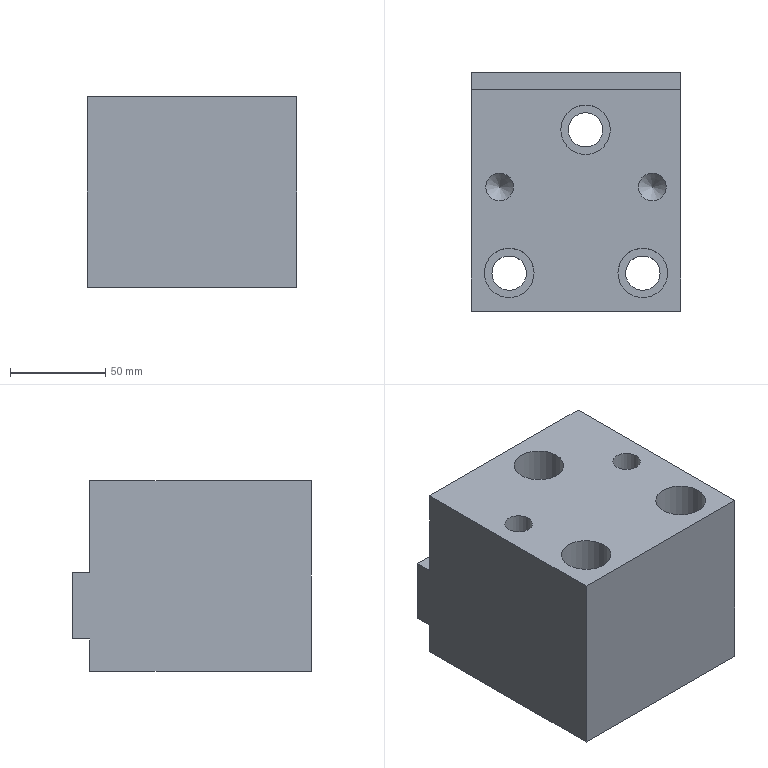Part | STEP file | lll_id4722_x_t | 1 solid | 27 faces | box 110 x 125 x 100 mm | volume 1169474 mm3 | plane 13 | cylinder 10 | cone 4 | commonest cylinder face diameters 18.009 x3 26.008 x3 8.5 x2 14.506 x2
STEP:
#1=CARTESIAN_POINT('',(1322.592,-417.359,5.));
#2=VERTEX_POINT('',#1);
#3=CARTESIAN_POINT('',(1315.339,-417.359,5.));
#4=DIRECTION('',(0.,0.,1.));
#5=DIRECTION('',(1.,0.,0.));
#6=AXIS2_PLACEMENT_3D('',#3,#4,#5);
#7=CIRCLE('',#6,7.253);
#8=EDGE_CURVE('',#2,#2,#7,.T.);
#9=ORIENTED_EDGE('',*,*,#8,.F.);
#10=EDGE_LOOP('',(#9));
#11=FACE_BOUND('',#10,.T.);
#12=CARTESIAN_POINT('',(1402.592,-417.359,5.));
#13=VERTEX_POINT('',#12);
#14=CARTESIAN_POINT('',(1395.339,-417.359,5.));
#15=DIRECTION('',(0.,0.,1.));
#16=DIRECTION('',(1.,0.,0.));
#17=AXIS2_PLACEMENT_3D('',#14,#15,#16);
#18=CIRCLE('',#17,7.253);
#19=EDGE_CURVE('',#13,#13,#18,.T.);
#20=ORIENTED_EDGE('',*,*,#19,.F.);
#21=EDGE_LOOP('',(#20));
#22=FACE_BOUND('',#21,.T.);
#23=CARTESIAN_POINT('',(1300.339,-366.359,5.));
#24=VERTEX_POINT('',#23);
#25=CARTESIAN_POINT('',(1410.339,-366.359,5.));
#26=VERTEX_POINT('',#25);
#27=CARTESIAN_POINT('',(-3297.001,-366.359,5.));
#28=DIRECTION('',(1.,0.,0.));
#29=VECTOR('',#28,1.);
#30=LINE('',#27,#29);
#31=EDGE_CURVE('',#24,#26,#30,.T.);
#32=ORIENTED_EDGE('',*,*,#31,.F.);
#33=CARTESIAN_POINT('',(1300.339,-482.359,5.));
#34=VERTEX_POINT('',#33);
#35=CARTESIAN_POINT('',(1300.339,-382.359,5.));
#36=DIRECTION('',(0.,-1.,0.));
#37=VECTOR('',#36,1.);
#38=LINE('',#35,#37);
#39=EDGE_CURVE('',#24,#34,#38,.T.);
#40=ORIENTED_EDGE('',*,*,#39,.T.);
#41=CARTESIAN_POINT('',(1410.339,-482.359,5.));
#42=VERTEX_POINT('',#41);
#43=CARTESIAN_POINT('',(1308.588,-482.359,5.));
#44=DIRECTION('',(-1.,0.,0.));
#45=VECTOR('',#44,1.);
#46=LINE('',#43,#45);
#47=EDGE_CURVE('',#42,#34,#46,.T.);
#48=ORIENTED_EDGE('',*,*,#47,.F.);
#49=CARTESIAN_POINT('',(1410.339,-382.359,5.));
#50=DIRECTION('',(0.,1.,0.));
#51=VECTOR('',#50,1.);
#52=LINE('',#49,#51);
#53=EDGE_CURVE('',#42,#26,#52,.T.);
#54=ORIENTED_EDGE('',*,*,#53,.T.);
#55=EDGE_LOOP('',(#32,#40,#48,#54));
#56=FACE_BOUND('',#55,.T.);
#57=CARTESIAN_POINT('',(1377.335,-462.359,5.));
#58=VERTEX_POINT('',#57);
#59=CARTESIAN_POINT('',(1390.339,-462.359,5.));
#60=DIRECTION('',(0.,0.,1.));
#61=DIRECTION('',(-1.,0.,0.));
#62=AXIS2_PLACEMENT_3D('',#59,#60,#61);
#63=CIRCLE('',#62,13.004);
#64=EDGE_CURVE('',#58,#58,#63,.T.);
#65=ORIENTED_EDGE('',*,*,#64,.F.);
#66=EDGE_LOOP('',(#65));
#67=FACE_BOUND('',#66,.T.);
#68=CARTESIAN_POINT('',(1307.335,-462.359,5.));
#69=VERTEX_POINT('',#68);
#70=CARTESIAN_POINT('',(1320.339,-462.359,5.));
#71=DIRECTION('',(0.,0.,1.));
#72=DIRECTION('',(-1.,0.,0.));
#73=AXIS2_PLACEMENT_3D('',#70,#71,#72);
#74=CIRCLE('',#73,13.004);
#75=EDGE_CURVE('',#69,#69,#74,.T.);
#76=ORIENTED_EDGE('',*,*,#75,.F.);
#77=EDGE_LOOP('',(#76));
#78=FACE_BOUND('',#77,.T.);
#79=CARTESIAN_POINT('',(1373.343,-387.359,5.));
#80=VERTEX_POINT('',#79);
#81=CARTESIAN_POINT('',(1360.339,-387.359,5.));
#82=DIRECTION('',(0.,0.,-1.));
#83=DIRECTION('',(1.,0.,0.));
#84=AXIS2_PLACEMENT_3D('',#81,#82,#83);
#85=CIRCLE('',#84,13.004);
#86=EDGE_CURVE('',#80,#80,#85,.T.);
#87=ORIENTED_EDGE('',*,*,#86,.T.);
#88=EDGE_LOOP('',(#87));
#89=FACE_BOUND('',#88,.T.);
#90=CARTESIAN_POINT('',(1308.588,-382.359,5.));
#91=DIRECTION('',(0.,0.,-1.));
#92=DIRECTION('',(1.,0.,0.));
#93=AXIS2_PLACEMENT_3D('',#90,#91,#92);
#94=PLANE('',#93);
#95=ADVANCED_FACE('',(#11,#22,#56,#67,#78,#89),#94,.F.);
#96=CARTESIAN_POINT('',(1330.339,-366.359,-23.25));
#97=VERTEX_POINT('',#96);
#98=CARTESIAN_POINT('',(1330.339,-366.359,-19.));
#99=DIRECTION('',(0.,-1.,0.));
#100=DIRECTION('',(0.,0.,-1.));
#101=AXIS2_PLACEMENT_3D('',#98,#99,#100);
#102=CIRCLE('',#101,4.25);
#103=EDGE_CURVE('',#97,#97,#102,.T.);
#104=ORIENTED_EDGE('',*,*,#103,.T.);
#105=EDGE_LOOP('',(#104));
#106=FACE_BOUND('',#105,.T.);
#107=CARTESIAN_POINT('',(1380.339,-366.359,-23.25));
#108=VERTEX_POINT('',#107);
#109=CARTESIAN_POINT('',(1380.339,-366.359,-19.));
#110=DIRECTION('',(0.,-1.,0.));
#111=DIRECTION('',(0.,0.,-1.));
#112=AXIS2_PLACEMENT_3D('',#109,#110,#111);
#113=CIRCLE('',#112,4.25);
#114=EDGE_CURVE('',#108,#108,#113,.T.);
#115=ORIENTED_EDGE('',*,*,#114,.T.);
#116=EDGE_LOOP('',(#115));
#117=FACE_BOUND('',#116,.T.);
#118=CARTESIAN_POINT('',(1300.339,-366.359,-43.));
#119=VERTEX_POINT('',#118);
#120=CARTESIAN_POINT('',(1410.339,-366.359,-43.));
#121=VERTEX_POINT('',#120);
#122=CARTESIAN_POINT('',(1305.339,-366.359,-43.));
#123=DIRECTION('',(1.,0.,0.));
#124=VECTOR('',#123,1.);
#125=LINE('',#122,#124);
#126=EDGE_CURVE('',#119,#121,#125,.T.);
#127=ORIENTED_EDGE('',*,*,#126,.F.);
#128=CARTESIAN_POINT('',(1300.339,-366.359,-625.));
#129=DIRECTION('',(0.,0.,-1.));
#130=VECTOR('',#129,1.);
#131=LINE('',#128,#130);
#132=EDGE_CURVE('',#24,#119,#131,.T.);
#133=ORIENTED_EDGE('',*,*,#132,.F.);
#134=ORIENTED_EDGE('',*,*,#31,.T.);
#135=CARTESIAN_POINT('',(1410.339,-366.359,-35.));
#136=DIRECTION('',(0.,0.,1.));
#137=VECTOR('',#136,1.);
#138=LINE('',#135,#137);
#139=EDGE_CURVE('',#121,#26,#138,.T.);
#140=ORIENTED_EDGE('',*,*,#139,.F.);
#141=EDGE_LOOP('',(#127,#133,#134,#140));
#142=FACE_BOUND('',#141,.T.);
#143=CARTESIAN_POINT('',(-3297.001,-366.359,-625.));
#144=DIRECTION('',(0.,1.,0.));
#145=DIRECTION('',(0.,0.,1.));
#146=AXIS2_PLACEMENT_3D('',#143,#144,#145);
#147=PLANE('',#146);
#148=ADVANCED_FACE('',(#106,#117,#142),#147,.T.);
#149=CARTESIAN_POINT('',(1300.339,-357.359,-78.));
#150=VERTEX_POINT('',#149);
#151=CARTESIAN_POINT('',(1300.339,-366.359,-78.));
#152=VERTEX_POINT('',#151);
#153=CARTESIAN_POINT('',(1300.339,-407.359,-78.));
#154=DIRECTION('',(0.,-1.,0.));
#155=VECTOR('',#154,1.);
#156=LINE('',#153,#155);
#157=EDGE_CURVE('',#150,#152,#156,.T.);
#158=ORIENTED_EDGE('',*,*,#157,.T.);
#159=CARTESIAN_POINT('',(1300.339,-366.359,-95.));
#160=VERTEX_POINT('',#159);
#161=CARTESIAN_POINT('',(1300.339,-366.359,72.5));
#162=DIRECTION('',(0.,0.,-1.));
#163=VECTOR('',#162,1.);
#164=LINE('',#161,#163);
#165=EDGE_CURVE('',#152,#160,#164,.T.);
#166=ORIENTED_EDGE('',*,*,#165,.T.);
#167=CARTESIAN_POINT('',(1300.339,-482.359,-95.));
#168=VERTEX_POINT('',#167);
#169=CARTESIAN_POINT('',(1300.339,-407.359,-95.));
#170=DIRECTION('',(0.,1.,0.));
#171=VECTOR('',#170,1.);
#172=LINE('',#169,#171);
#173=EDGE_CURVE('',#168,#160,#172,.T.);
#174=ORIENTED_EDGE('',*,*,#173,.F.);
#175=CARTESIAN_POINT('',(1300.339,-482.359,-650.));
#176=DIRECTION('',(0.,0.,-1.));
#177=VECTOR('',#176,1.);
#178=LINE('',#175,#177);
#179=EDGE_CURVE('',#34,#168,#178,.T.);
#180=ORIENTED_EDGE('',*,*,#179,.F.);
#181=ORIENTED_EDGE('',*,*,#39,.F.);
#182=ORIENTED_EDGE('',*,*,#132,.T.);
#183=CARTESIAN_POINT('',(1300.339,-357.359,-43.));
#184=VERTEX_POINT('',#183);
#185=CARTESIAN_POINT('',(1300.339,-397.359,-43.));
#186=DIRECTION('',(0.,1.,0.));
#187=VECTOR('',#186,1.);
#188=LINE('',#185,#187);
#189=EDGE_CURVE('',#119,#184,#188,.T.);
#190=ORIENTED_EDGE('',*,*,#189,.T.);
#191=CARTESIAN_POINT('',(1300.339,-357.359,72.5));
#192=DIRECTION('',(0.,0.,-1.));
#193=VECTOR('',#192,1.);
#194=LINE('',#191,#193);
#195=EDGE_CURVE('',#184,#150,#194,.T.);
#196=ORIENTED_EDGE('',*,*,#195,.T.);
#197=EDGE_LOOP('',(#158,#166,#174,#180,#181,#182,#190,#196));
#198=FACE_OUTER_BOUND('',#197,.T.);
#199=CARTESIAN_POINT('',(1300.339,-407.359,72.5));
#200=DIRECTION('',(-1.,0.,0.));
#201=DIRECTION('',(0.,0.,-1.));
#202=AXIS2_PLACEMENT_3D('',#199,#200,#201);
#203=PLANE('',#202);
#204=ADVANCED_FACE('',(#198),#203,.T.);
#205=CARTESIAN_POINT('',(1410.339,-357.359,-78.));
#206=VERTEX_POINT('',#205);
#207=CARTESIAN_POINT('',(-3297.001,-357.359,-78.));
#208=DIRECTION('',(1.,0.,0.));
#209=VECTOR('',#208,1.);
#210=LINE('',#207,#209);
#211=EDGE_CURVE('',#150,#206,#210,.T.);
#212=ORIENTED_EDGE('',*,*,#211,.F.);
#213=ORIENTED_EDGE('',*,*,#195,.F.);
#214=CARTESIAN_POINT('',(1410.339,-357.359,-43.));
#215=VERTEX_POINT('',#214);
#216=CARTESIAN_POINT('',(-3297.001,-357.359,-43.));
#217=DIRECTION('',(-1.,0.,0.));
#218=VECTOR('',#217,1.);
#219=LINE('',#216,#218);
#220=EDGE_CURVE('',#215,#184,#219,.T.);
#221=ORIENTED_EDGE('',*,*,#220,.F.);
#222=CARTESIAN_POINT('',(1410.339,-357.359,-60.));
#223=DIRECTION('',(0.,0.,1.));
#224=VECTOR('',#223,1.);
#225=LINE('',#222,#224);
#226=EDGE_CURVE('',#206,#215,#225,.T.);
#227=ORIENTED_EDGE('',*,*,#226,.F.);
#228=EDGE_LOOP('',(#212,#213,#221,#227));
#229=FACE_OUTER_BOUND('',#228,.T.);
#230=CARTESIAN_POINT('',(-3297.001,-357.359,-650.));
#231=DIRECTION('',(0.,1.,0.));
#232=DIRECTION('',(0.,0.,1.));
#233=AXIS2_PLACEMENT_3D('',#230,#231,#232);
#234=PLANE('',#233);
#235=ADVANCED_FACE('',(#229),#234,.T.);
#236=ORIENTED_EDGE('',*,*,#179,.T.);
#237=CARTESIAN_POINT('',(1410.339,-482.359,-95.));
#238=VERTEX_POINT('',#237);
#239=CARTESIAN_POINT('',(-3297.001,-482.359,-95.));
#240=DIRECTION('',(1.,0.,0.));
#241=VECTOR('',#240,1.);
#242=LINE('',#239,#241);
#243=EDGE_CURVE('',#168,#238,#242,.T.);
#244=ORIENTED_EDGE('',*,*,#243,.T.);
#245=CARTESIAN_POINT('',(1410.339,-482.359,-650.));
#246=DIRECTION('',(0.,0.,-1.));
#247=VECTOR('',#246,1.);
#248=LINE('',#245,#247);
#249=EDGE_CURVE('',#42,#238,#248,.T.);
#250=ORIENTED_EDGE('',*,*,#249,.F.);
#251=ORIENTED_EDGE('',*,*,#47,.T.);
#252=EDGE_LOOP('',(#236,#244,#250,#251));
#253=FACE_OUTER_BOUND('',#252,.T.);
#254=CARTESIAN_POINT('',(-3297.001,-482.359,-650.));
#255=DIRECTION('',(0.,1.,0.));
#256=DIRECTION('',(0.,0.,1.));
#257=AXIS2_PLACEMENT_3D('',#254,#255,#256);
#258=PLANE('',#257);
#259=ADVANCED_FACE('',(#253),#258,.F.);
#260=ORIENTED_EDGE('',*,*,#249,.T.);
#261=CARTESIAN_POINT('',(1410.339,-366.359,-95.));
#262=VERTEX_POINT('',#261);
#263=CARTESIAN_POINT('',(1410.339,-233.52,-95.));
#264=DIRECTION('',(0.,-1.,0.));
#265=VECTOR('',#264,1.);
#266=LINE('',#263,#265);
#267=EDGE_CURVE('',#262,#238,#266,.T.);
#268=ORIENTED_EDGE('',*,*,#267,.F.);
#269=CARTESIAN_POINT('',(1410.339,-366.359,-78.));
#270=VERTEX_POINT('',#269);
#271=CARTESIAN_POINT('',(1410.339,-366.359,-650.));
#272=DIRECTION('',(0.,0.,1.));
#273=VECTOR('',#272,1.);
#274=LINE('',#271,#273);
#275=EDGE_CURVE('',#262,#270,#274,.T.);
#276=ORIENTED_EDGE('',*,*,#275,.T.);
#277=CARTESIAN_POINT('',(1410.339,-382.359,-78.));
#278=DIRECTION('',(0.,1.,0.));
#279=VECTOR('',#278,1.);
#280=LINE('',#277,#279);
#281=EDGE_CURVE('',#270,#206,#280,.T.);
#282=ORIENTED_EDGE('',*,*,#281,.T.);
#283=ORIENTED_EDGE('',*,*,#226,.T.);
#284=CARTESIAN_POINT('',(1410.339,-382.359,-43.));
#285=DIRECTION('',(0.,-1.,0.));
#286=VECTOR('',#285,1.);
#287=LINE('',#284,#286);
#288=EDGE_CURVE('',#215,#121,#287,.T.);
#289=ORIENTED_EDGE('',*,*,#288,.T.);
#290=ORIENTED_EDGE('',*,*,#139,.T.);
#291=ORIENTED_EDGE('',*,*,#53,.F.);
#292=EDGE_LOOP('',(#260,#268,#276,#282,#283,#289,#290,#291));
#293=FACE_OUTER_BOUND('',#292,.T.);
#294=CARTESIAN_POINT('',(1410.339,-382.359,-60.));
#295=DIRECTION('',(-1.,0.,0.));
#296=DIRECTION('',(0.,0.,-1.));
#297=AXIS2_PLACEMENT_3D('',#294,#295,#296);
#298=PLANE('',#297);
#299=ADVANCED_FACE('',(#293),#298,.F.);
#300=ORIENTED_EDGE('',*,*,#126,.T.);
#301=ORIENTED_EDGE('',*,*,#288,.F.);
#302=ORIENTED_EDGE('',*,*,#220,.T.);
#303=ORIENTED_EDGE('',*,*,#189,.F.);
#304=EDGE_LOOP('',(#300,#301,#302,#303));
#305=FACE_OUTER_BOUND('',#304,.T.);
#306=CARTESIAN_POINT('',(1305.339,-397.359,-43.));
#307=DIRECTION('',(0.,0.,1.));
#308=DIRECTION('',(-1.,0.,0.));
#309=AXIS2_PLACEMENT_3D('',#306,#307,#308);
#310=PLANE('',#309);
#311=ADVANCED_FACE('',(#305),#310,.T.);
#312=CARTESIAN_POINT('',(1399.344,-462.359,-55.));
#313=VERTEX_POINT('',#312);
#314=CARTESIAN_POINT('',(1390.339,-462.359,-55.));
#315=DIRECTION('',(0.,0.,1.));
#316=DIRECTION('',(1.,0.,0.));
#317=AXIS2_PLACEMENT_3D('',#314,#315,#316);
#318=CIRCLE('',#317,9.005);
#319=EDGE_CURVE('',#313,#313,#318,.T.);
#320=ORIENTED_EDGE('',*,*,#319,.T.);
#321=EDGE_LOOP('',(#320));
#322=FACE_BOUND('',#321,.T.);
#323=CARTESIAN_POINT('',(1399.344,-462.359,-95.));
#324=VERTEX_POINT('',#323);
#325=CARTESIAN_POINT('',(1390.339,-462.359,-95.));
#326=DIRECTION('',(0.,0.,1.));
#327=DIRECTION('',(1.,0.,0.));
#328=AXIS2_PLACEMENT_3D('',#325,#326,#327);
#329=CIRCLE('',#328,9.005);
#330=EDGE_CURVE('',#324,#324,#329,.T.);
#331=ORIENTED_EDGE('',*,*,#330,.F.);
#332=EDGE_LOOP('',(#331));
#333=FACE_BOUND('',#332,.T.);
#334=CARTESIAN_POINT('',(1390.339,-462.359,-18.));
#335=DIRECTION('',(0.,0.,-1.));
#336=DIRECTION('',(-1.,0.,0.));
#337=AXIS2_PLACEMENT_3D('',#334,#335,#336);
#338=CYLINDRICAL_SURFACE('',#337,9.005);
#339=ADVANCED_FACE('',(#322,#333),#338,.F.);
#340=ORIENTED_EDGE('',*,*,#319,.F.);
#341=EDGE_LOOP('',(#340));
#342=FACE_BOUND('',#341,.T.);
#343=CARTESIAN_POINT('',(1377.335,-462.359,-55.));
#344=VERTEX_POINT('',#343);
#345=CARTESIAN_POINT('',(1390.339,-462.359,-55.));
#346=DIRECTION('',(0.,0.,1.));
#347=DIRECTION('',(-1.,0.,0.));
#348=AXIS2_PLACEMENT_3D('',#345,#346,#347);
#349=CIRCLE('',#348,13.004);
#350=EDGE_CURVE('',#344,#344,#349,.T.);
#351=ORIENTED_EDGE('',*,*,#350,.T.);
#352=EDGE_LOOP('',(#351));
#353=FACE_BOUND('',#352,.T.);
#354=CARTESIAN_POINT('',(1390.339,-462.359,-55.));
#355=DIRECTION('',(0.,0.,-1.));
#356=DIRECTION('',(1.,0.,0.));
#357=AXIS2_PLACEMENT_3D('',#354,#355,#356);
#358=PLANE('',#357);
#359=ADVANCED_FACE('',(#342,#353),#358,.F.);
#360=ORIENTED_EDGE('',*,*,#350,.F.);
#361=EDGE_LOOP('',(#360));
#362=FACE_BOUND('',#361,.T.);
#363=ORIENTED_EDGE('',*,*,#64,.T.);
#364=EDGE_LOOP('',(#363));
#365=FACE_BOUND('',#364,.T.);
#366=CARTESIAN_POINT('',(1390.339,-462.359,5.));
#367=DIRECTION('',(0.,0.,-1.));
#368=DIRECTION('',(-1.,0.,0.));
#369=AXIS2_PLACEMENT_3D('',#366,#367,#368);
#370=CYLINDRICAL_SURFACE('',#369,13.004);
#371=ADVANCED_FACE('',(#362,#365),#370,.F.);
#372=CARTESIAN_POINT('',(1329.344,-462.359,-55.));
#373=VERTEX_POINT('',#372);
#374=CARTESIAN_POINT('',(1320.339,-462.359,-55.));
#375=DIRECTION('',(0.,0.,1.));
#376=DIRECTION('',(1.,0.,0.));
#377=AXIS2_PLACEMENT_3D('',#374,#375,#376);
#378=CIRCLE('',#377,9.005);
#379=EDGE_CURVE('',#373,#373,#378,.T.);
#380=ORIENTED_EDGE('',*,*,#379,.T.);
#381=EDGE_LOOP('',(#380));
#382=FACE_BOUND('',#381,.T.);
#383=CARTESIAN_POINT('',(1329.344,-462.359,-95.));
#384=VERTEX_POINT('',#383);
#385=CARTESIAN_POINT('',(1320.339,-462.359,-95.));
#386=DIRECTION('',(0.,0.,1.));
#387=DIRECTION('',(1.,0.,0.));
#388=AXIS2_PLACEMENT_3D('',#385,#386,#387);
#389=CIRCLE('',#388,9.005);
#390=EDGE_CURVE('',#384,#384,#389,.T.);
#391=ORIENTED_EDGE('',*,*,#390,.F.);
#392=EDGE_LOOP('',(#391));
#393=FACE_BOUND('',#392,.T.);
#394=CARTESIAN_POINT('',(1320.339,-462.359,-18.));
#395=DIRECTION('',(0.,0.,-1.));
#396=DIRECTION('',(-1.,0.,0.));
#397=AXIS2_PLACEMENT_3D('',#394,#395,#396);
#398=CYLINDRICAL_SURFACE('',#397,9.005);
#399=ADVANCED_FACE('',(#382,#393),#398,.F.);
#400=ORIENTED_EDGE('',*,*,#379,.F.);
#401=EDGE_LOOP('',(#400));
#402=FACE_BOUND('',#401,.T.);
#403=CARTESIAN_POINT('',(1307.335,-462.359,-55.));
#404=VERTEX_POINT('',#403);
#405=CARTESIAN_POINT('',(1320.339,-462.359,-55.));
#406=DIRECTION('',(0.,0.,1.));
#407=DIRECTION('',(-1.,0.,0.));
#408=AXIS2_PLACEMENT_3D('',#405,#406,#407);
#409=CIRCLE('',#408,13.004);
#410=EDGE_CURVE('',#404,#404,#409,.T.);
#411=ORIENTED_EDGE('',*,*,#410,.T.);
#412=EDGE_LOOP('',(#411));
#413=FACE_BOUND('',#412,.T.);
#414=CARTESIAN_POINT('',(1320.339,-462.359,-55.));
#415=DIRECTION('',(0.,0.,-1.));
#416=DIRECTION('',(1.,0.,0.));
#417=AXIS2_PLACEMENT_3D('',#414,#415,#416);
#418=PLANE('',#417);
#419=ADVANCED_FACE('',(#402,#413),#418,.F.);
#420=ORIENTED_EDGE('',*,*,#410,.F.);
#421=EDGE_LOOP('',(#420));
#422=FACE_BOUND('',#421,.T.);
#423=ORIENTED_EDGE('',*,*,#75,.T.);
#424=EDGE_LOOP('',(#423));
#425=FACE_BOUND('',#424,.T.);
#426=CARTESIAN_POINT('',(1320.339,-462.359,5.));
#427=DIRECTION('',(0.,0.,-1.));
#428=DIRECTION('',(-1.,0.,0.));
#429=AXIS2_PLACEMENT_3D('',#426,#427,#428);
#430=CYLINDRICAL_SURFACE('',#429,13.004);
#431=ADVANCED_FACE('',(#422,#425),#430,.F.);
#432=CARTESIAN_POINT('',(1351.335,-387.359,-55.));
#433=VERTEX_POINT('',#432);
#434=CARTESIAN_POINT('',(1360.339,-387.359,-55.));
#435=DIRECTION('',(0.,0.,-1.));
#436=DIRECTION('',(-1.,0.,0.));
#437=AXIS2_PLACEMENT_3D('',#434,#435,#436);
#438=CIRCLE('',#437,9.005);
#439=EDGE_CURVE('',#433,#433,#438,.T.);
#440=ORIENTED_EDGE('',*,*,#439,.F.);
#441=EDGE_LOOP('',(#440));
#442=FACE_BOUND('',#441,.T.);
#443=CARTESIAN_POINT('',(1369.344,-387.359,-95.));
#444=VERTEX_POINT('',#443);
#445=CARTESIAN_POINT('',(1360.339,-387.359,-95.));
#446=DIRECTION('',(0.,0.,1.));
#447=DIRECTION('',(1.,0.,0.));
#448=AXIS2_PLACEMENT_3D('',#445,#446,#447);
#449=CIRCLE('',#448,9.005);
#450=EDGE_CURVE('',#444,#444,#449,.T.);
#451=ORIENTED_EDGE('',*,*,#450,.F.);
#452=EDGE_LOOP('',(#451));
#453=FACE_BOUND('',#452,.T.);
#454=CARTESIAN_POINT('',(1360.339,-387.359,-18.));
#455=DIRECTION('',(0.,0.,-1.));
#456=DIRECTION('',(1.,0.,0.));
#457=AXIS2_PLACEMENT_3D('',#454,#455,#456);
#458=CYLINDRICAL_SURFACE('',#457,9.005);
#459=ADVANCED_FACE('',(#442,#453),#458,.F.);
#460=ORIENTED_EDGE('',*,*,#439,.T.);
#461=EDGE_LOOP('',(#460));
#462=FACE_BOUND('',#461,.T.);
#463=CARTESIAN_POINT('',(1373.343,-387.359,-55.));
#464=VERTEX_POINT('',#463);
#465=CARTESIAN_POINT('',(1360.339,-387.359,-55.));
#466=DIRECTION('',(0.,0.,-1.));
#467=DIRECTION('',(-1.,0.,0.));
#468=AXIS2_PLACEMENT_3D('',#465,#466,#467);
#469=CIRCLE('',#468,13.004);
#470=EDGE_CURVE('',#464,#464,#469,.T.);
#471=ORIENTED_EDGE('',*,*,#470,.F.);
#472=EDGE_LOOP('',(#471));
#473=FACE_BOUND('',#472,.T.);
#474=CARTESIAN_POINT('',(1360.339,-387.359,-55.));
#475=DIRECTION('',(0.,0.,-1.));
#476=DIRECTION('',(-1.,0.,0.));
#477=AXIS2_PLACEMENT_3D('',#474,#475,#476);
#478=PLANE('',#477);
#479=ADVANCED_FACE('',(#462,#473),#478,.F.);
#480=ORIENTED_EDGE('',*,*,#470,.T.);
#481=EDGE_LOOP('',(#480));
#482=FACE_BOUND('',#481,.T.);
#483=ORIENTED_EDGE('',*,*,#86,.F.);
#484=EDGE_LOOP('',(#483));
#485=FACE_BOUND('',#484,.T.);
#486=CARTESIAN_POINT('',(1360.339,-387.359,5.));
#487=DIRECTION('',(0.,0.,-1.));
#488=DIRECTION('',(1.,0.,0.));
#489=AXIS2_PLACEMENT_3D('',#486,#487,#488);
#490=CYLINDRICAL_SURFACE('',#489,13.004);
#491=ADVANCED_FACE('',(#482,#485),#490,.F.);
#492=CARTESIAN_POINT('',(1402.592,-417.359,-30.753));
#493=VERTEX_POINT('',#492);
#494=CARTESIAN_POINT('',(1395.339,-417.359,-30.753));
#495=DIRECTION('',(0.,0.,1.));
#496=DIRECTION('',(1.,0.,0.));
#497=AXIS2_PLACEMENT_3D('',#494,#495,#496);
#498=CIRCLE('',#497,7.253);
#499=EDGE_CURVE('',#493,#493,#498,.T.);
#500=ORIENTED_EDGE('',*,*,#499,.F.);
#501=EDGE_LOOP('',(#500));
#502=FACE_BOUND('',#501,.T.);
#503=ORIENTED_EDGE('',*,*,#19,.T.);
#504=EDGE_LOOP('',(#503));
#505=FACE_BOUND('',#504,.T.);
#506=CARTESIAN_POINT('',(1395.339,-417.359,7.));
#507=DIRECTION('',(0.,0.,-1.));
#508=DIRECTION('',(-1.,0.,0.));
#509=AXIS2_PLACEMENT_3D('',#506,#507,#508);
#510=CYLINDRICAL_SURFACE('',#509,7.253);
#511=ADVANCED_FACE('',(#502,#505),#510,.F.);
#512=CARTESIAN_POINT('',(1395.339,-417.359,-38.006));
#513=VERTEX_POINT('',#512);
#514=VERTEX_LOOP('',#513);
#515=FACE_BOUND('',#514,.T.);
#516=ORIENTED_EDGE('',*,*,#499,.T.);
#517=EDGE_LOOP('',(#516));
#518=FACE_BOUND('',#517,.T.);
#519=CARTESIAN_POINT('',(1395.339,-417.359,-30.753));
#520=DIRECTION('',(0.,0.,1.));
#521=DIRECTION('',(-1.,0.,0.));
#522=AXIS2_PLACEMENT_3D('',#519,#520,#521);
#523=CONICAL_SURFACE('',#522,7.253,45.);
#524=ADVANCED_FACE('',(#515,#518),#523,.F.);
#525=CARTESIAN_POINT('',(1308.086,-417.359,-30.753));
#526=VERTEX_POINT('',#525);
#527=CARTESIAN_POINT('',(1315.339,-417.359,-30.753));
#528=DIRECTION('',(0.,0.,-1.));
#529=DIRECTION('',(-1.,0.,0.));
#530=AXIS2_PLACEMENT_3D('',#527,#528,#529);
#531=CIRCLE('',#530,7.253);
#532=EDGE_CURVE('',#526,#526,#531,.T.);
#533=ORIENTED_EDGE('',*,*,#532,.T.);
#534=EDGE_LOOP('',(#533));
#535=FACE_BOUND('',#534,.T.);
#536=ORIENTED_EDGE('',*,*,#8,.T.);
#537=EDGE_LOOP('',(#536));
#538=FACE_BOUND('',#537,.T.);
#539=CARTESIAN_POINT('',(1315.339,-417.359,7.));
#540=DIRECTION('',(0.,0.,-1.));
#541=DIRECTION('',(1.,0.,0.));
#542=AXIS2_PLACEMENT_3D('',#539,#540,#541);
#543=CYLINDRICAL_SURFACE('',#542,7.253);
#544=ADVANCED_FACE('',(#535,#538),#543,.F.);
#545=CARTESIAN_POINT('',(1315.339,-417.359,-38.006));
#546=VERTEX_POINT('',#545);
#547=VERTEX_LOOP('',#546);
#548=FACE_BOUND('',#547,.T.);
#549=ORIENTED_EDGE('',*,*,#532,.F.);
#550=EDGE_LOOP('',(#549));
#551=FACE_BOUND('',#550,.T.);
#552=CARTESIAN_POINT('',(1315.339,-417.359,-30.753));
#553=DIRECTION('',(0.,0.,1.));
#554=DIRECTION('',(1.,0.,0.));
#555=AXIS2_PLACEMENT_3D('',#552,#553,#554);
#556=CONICAL_SURFACE('',#555,7.253,45.);
#557=ADVANCED_FACE('',(#548,#551),#556,.F.);
#558=CARTESIAN_POINT('',(1380.339,-386.359,-23.25));
#559=VERTEX_POINT('',#558);
#560=CARTESIAN_POINT('',(1380.339,-386.359,-19.));
#561=DIRECTION('',(0.,1.,0.));
#562=DIRECTION('',(0.,0.,-1.));
#563=AXIS2_PLACEMENT_3D('',#560,#561,#562);
#564=CIRCLE('',#563,4.25);
#565=EDGE_CURVE('',#559,#559,#564,.T.);
#566=ORIENTED_EDGE('',*,*,#565,.T.);
#567=EDGE_LOOP('',(#566));
#568=FACE_BOUND('',#567,.T.);
#569=CARTESIAN_POINT('',(1380.339,-388.913,-19.));
#570=VERTEX_POINT('',#569);
#571=VERTEX_LOOP('',#570);
#572=FACE_BOUND('',#571,.T.);
#573=CARTESIAN_POINT('',(1380.339,-386.359,-19.));
#574=DIRECTION('',(0.,1.,0.));
#575=DIRECTION('',(0.,0.,1.));
#576=AXIS2_PLACEMENT_3D('',#573,#574,#575);
#577=CONICAL_SURFACE('',#576,4.25,59.);
#578=ADVANCED_FACE('',(#568,#572),#577,.F.);
#579=ORIENTED_EDGE('',*,*,#565,.F.);
#580=EDGE_LOOP('',(#579));
#581=FACE_BOUND('',#580,.T.);
#582=ORIENTED_EDGE('',*,*,#114,.F.);
#583=EDGE_LOOP('',(#582));
#584=FACE_BOUND('',#583,.T.);
#585=CARTESIAN_POINT('',(1380.339,-366.359,-19.));
#586=DIRECTION('',(0.,-1.,0.));
#587=DIRECTION('',(0.,0.,-1.));
#588=AXIS2_PLACEMENT_3D('',#585,#586,#587);
#589=CYLINDRICAL_SURFACE('',#588,4.25);
#590=ADVANCED_FACE('',(#581,#584),#589,.F.);
#591=CARTESIAN_POINT('',(1330.339,-386.359,-23.25));
#592=VERTEX_POINT('',#591);
#593=CARTESIAN_POINT('',(1330.339,-386.359,-19.));
#594=DIRECTION('',(0.,1.,0.));
#595=DIRECTION('',(0.,0.,-1.));
#596=AXIS2_PLACEMENT_3D('',#593,#594,#595);
#597=CIRCLE('',#596,4.25);
#598=EDGE_CURVE('',#592,#592,#597,.T.);
#599=ORIENTED_EDGE('',*,*,#598,.T.);
#600=EDGE_LOOP('',(#599));
#601=FACE_BOUND('',#600,.T.);
#602=CARTESIAN_POINT('',(1330.339,-388.913,-19.));
#603=VERTEX_POINT('',#602);
#604=VERTEX_LOOP('',#603);
#605=FACE_BOUND('',#604,.T.);
#606=CARTESIAN_POINT('',(1330.339,-386.359,-19.));
#607=DIRECTION('',(0.,1.,0.));
#608=DIRECTION('',(0.,0.,1.));
#609=AXIS2_PLACEMENT_3D('',#606,#607,#608);
#610=CONICAL_SURFACE('',#609,4.25,59.);
#611=ADVANCED_FACE('',(#601,#605),#610,.F.);
#612=ORIENTED_EDGE('',*,*,#598,.F.);
#613=EDGE_LOOP('',(#612));
#614=FACE_BOUND('',#613,.T.);
#615=ORIENTED_EDGE('',*,*,#103,.F.);
#616=EDGE_LOOP('',(#615));
#617=FACE_BOUND('',#616,.T.);
#618=CARTESIAN_POINT('',(1330.339,-366.359,-19.));
#619=DIRECTION('',(0.,-1.,0.));
#620=DIRECTION('',(0.,0.,-1.));
#621=AXIS2_PLACEMENT_3D('',#618,#619,#620);
#622=CYLINDRICAL_SURFACE('',#621,4.25);
#623=ADVANCED_FACE('',(#614,#617),#622,.F.);
#624=ORIENTED_EDGE('',*,*,#281,.F.);
#625=CARTESIAN_POINT('',(2067.435,-366.359,-78.));
#626=DIRECTION('',(-1.,0.,0.));
#627=VECTOR('',#626,1.);
#628=LINE('',#625,#627);
#629=EDGE_CURVE('',#270,#152,#628,.T.);
#630=ORIENTED_EDGE('',*,*,#629,.T.);
#631=ORIENTED_EDGE('',*,*,#157,.F.);
#632=ORIENTED_EDGE('',*,*,#211,.T.);
#633=EDGE_LOOP('',(#624,#630,#631,#632));
#634=FACE_OUTER_BOUND('',#633,.T.);
#635=CARTESIAN_POINT('',(2067.435,0.000000688,-78.));
#636=DIRECTION('',(0.,0.,1.));
#637=DIRECTION('',(-1.,0.,0.));
#638=AXIS2_PLACEMENT_3D('',#635,#636,#637);
#639=PLANE('',#638);
#640=ADVANCED_FACE('',(#634),#639,.F.);
#641=ORIENTED_EDGE('',*,*,#165,.F.);
#642=ORIENTED_EDGE('',*,*,#629,.F.);
#643=ORIENTED_EDGE('',*,*,#275,.F.);
#644=CARTESIAN_POINT('',(1554.249,-366.359,-95.));
#645=DIRECTION('',(1.,0.,0.));
#646=VECTOR('',#645,1.);
#647=LINE('',#644,#646);
#648=EDGE_CURVE('',#160,#262,#647,.T.);
#649=ORIENTED_EDGE('',*,*,#648,.F.);
#650=EDGE_LOOP('',(#641,#642,#643,#649));
#651=FACE_OUTER_BOUND('',#650,.T.);
#652=CARTESIAN_POINT('',(-3297.001,-366.359,-650.));
#653=DIRECTION('',(0.,1.,0.));
#654=DIRECTION('',(0.,0.,1.));
#655=AXIS2_PLACEMENT_3D('',#652,#653,#654);
#656=PLANE('',#655);
#657=ADVANCED_FACE('',(#651),#656,.T.);
#658=ORIENTED_EDGE('',*,*,#450,.T.);
#659=EDGE_LOOP('',(#658));
#660=FACE_BOUND('',#659,.T.);
#661=ORIENTED_EDGE('',*,*,#390,.T.);
#662=EDGE_LOOP('',(#661));
#663=FACE_BOUND('',#662,.T.);
#664=ORIENTED_EDGE('',*,*,#330,.T.);
#665=EDGE_LOOP('',(#664));
#666=FACE_BOUND('',#665,.T.);
#667=ORIENTED_EDGE('',*,*,#267,.T.);
#668=ORIENTED_EDGE('',*,*,#243,.F.);
#669=ORIENTED_EDGE('',*,*,#173,.T.);
#670=ORIENTED_EDGE('',*,*,#648,.T.);
#671=EDGE_LOOP('',(#667,#668,#669,#670));
#672=FACE_BOUND('',#671,.T.);
#673=CARTESIAN_POINT('',(1554.249,-233.52,-95.));
#674=DIRECTION('',(0.,0.,-1.));
#675=DIRECTION('',(1.,0.,0.));
#676=AXIS2_PLACEMENT_3D('',#673,#674,#675);
#677=PLANE('',#676);
#678=ADVANCED_FACE('',(#660,#663,#666,#672),#677,.T.);
#679=CLOSED_SHELL('',(#95,#148,#204,#235,#259,#299,#311,#339,#359,#371,#399,#419,#431,#459,#479,#491,#511,#524,#544,#557,#578,#590,#611,#623,#640,#657,#678));
#680=MANIFOLD_SOLID_BREP('',#679);
#681=(LENGTH_UNIT()NAMED_UNIT(*)SI_UNIT(.MILLI.,.METRE.));
#682=UNCERTAINTY_MEASURE_WITH_UNIT(LENGTH_MEASURE(0.00002),#681,'','');
#683=(NAMED_UNIT(*)PLANE_ANGLE_UNIT()SI_UNIT($,.RADIAN.));
#684=PLANE_ANGLE_MEASURE_WITH_UNIT(PLANE_ANGLE_MEASURE(0.01745),#683);
#685=DIMENSIONAL_EXPONENTS(0.,0.,0.,0.,0.,0.,0.);
#686=(CONVERSION_BASED_UNIT('DEGREE',#684)NAMED_UNIT(#685)PLANE_ANGLE_UNIT());
#687=(NAMED_UNIT(*)SI_UNIT($,.STERADIAN.)SOLID_ANGLE_UNIT());
#688=(GEOMETRIC_REPRESENTATION_CONTEXT(3)GLOBAL_UNCERTAINTY_ASSIGNED_CONTEXT((#682))GLOBAL_UNIT_ASSIGNED_CONTEXT((#681,#686,#687))REPRESENTATION_CONTEXT('',''));
#689=ADVANCED_BREP_SHAPE_REPRESENTATION('',(#680),#688);